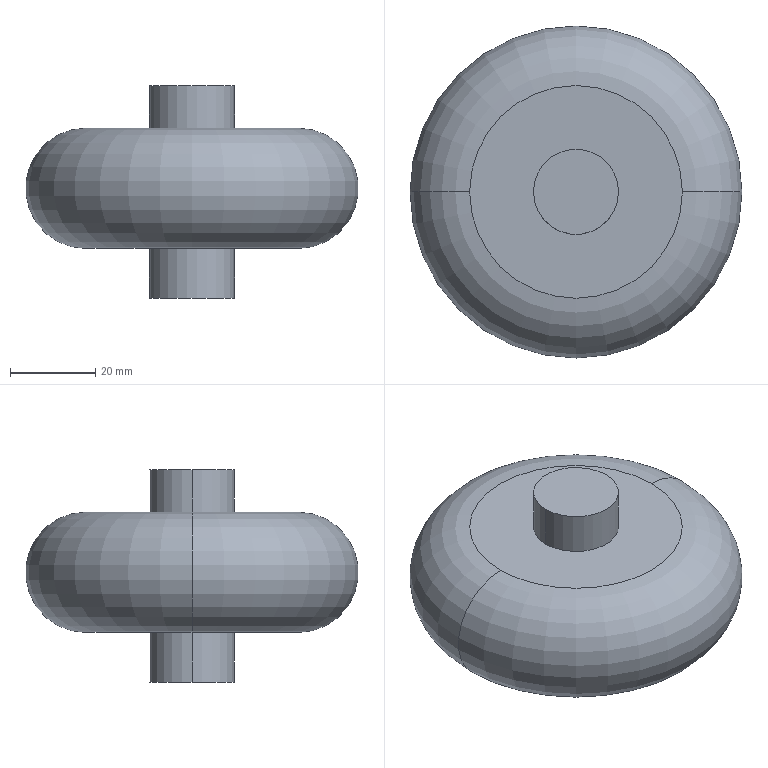Part | SolidWorks | features Extrusion 1, Revolution 1 | 1 solid | 10 faces | box 78.234 x 78.234 x 50 mm | volume 123364 mm3 | cylinder 4 | plane 4 | torus 2 | commonest cylinder face diameters 20 x4
STEP:
#1=CARTESIAN_POINT('',(10.,0.,25.));
#2=VERTEX_POINT('',#1);
#3=CARTESIAN_POINT('',(-10.,0.,25.));
#4=VERTEX_POINT('',#3);
#5=CARTESIAN_POINT('',(0.,0.,25.));
#6=DIRECTION('',(0.,0.,1.));
#7=DIRECTION('',(1.,0.,0.));
#8=AXIS2_PLACEMENT_3D('',#5,#6,#7);
#9=CIRCLE('',#8,10.);
#10=EDGE_CURVE('',#2,#4,#9,.T.);
#11=ORIENTED_EDGE('',*,*,#10,.F.);
#12=CARTESIAN_POINT('',(10.,0.,15.));
#13=VERTEX_POINT('',#12);
#14=CARTESIAN_POINT('',(10.,0.,25.));
#15=DIRECTION('',(0.,0.,-1.));
#16=VECTOR('',#15,1000.);
#17=LINE('',#14,#16);
#18=EDGE_CURVE('',#2,#13,#17,.T.);
#19=ORIENTED_EDGE('',*,*,#18,.T.);
#20=CARTESIAN_POINT('',(-10.,0.,15.));
#21=VERTEX_POINT('',#20);
#22=CARTESIAN_POINT('',(0.,0.,15.));
#23=DIRECTION('',(0.,0.,-1.));
#24=DIRECTION('',(-1.,0.,0.));
#25=AXIS2_PLACEMENT_3D('',#22,#23,#24);
#26=CIRCLE('',#25,10.);
#27=EDGE_CURVE('',#21,#13,#26,.T.);
#28=ORIENTED_EDGE('',*,*,#27,.F.);
#29=CARTESIAN_POINT('',(-10.,0.,25.));
#30=DIRECTION('',(0.,0.,-1.));
#31=VECTOR('',#30,1000.);
#32=LINE('',#29,#31);
#33=EDGE_CURVE('',#4,#21,#32,.T.);
#34=ORIENTED_EDGE('',*,*,#33,.F.);
#35=EDGE_LOOP('',(#11,#19,#28,#34));
#36=FACE_OUTER_BOUND('',#35,.T.);
#37=CARTESIAN_POINT('',(0.,0.,25.));
#38=DIRECTION('',(0.,0.,-1.));
#39=DIRECTION('',(-1.,0.,0.));
#40=AXIS2_PLACEMENT_3D('',#37,#38,#39);
#41=CYLINDRICAL_SURFACE('',#40,10.);
#42=ADVANCED_FACE('',(#36),#41,.T.);
#43=CARTESIAN_POINT('',(-24.991,0.,15.));
#44=VERTEX_POINT('',#43);
#45=CARTESIAN_POINT('',(24.991,0.,15.));
#46=VERTEX_POINT('',#45);
#47=CARTESIAN_POINT('',(-0.000000001,0.,15.));
#48=DIRECTION('',(0.,0.,-1.));
#49=DIRECTION('',(-1.,0.,0.));
#50=AXIS2_PLACEMENT_3D('',#47,#48,#49);
#51=CIRCLE('',#50,24.991);
#52=EDGE_CURVE('',#44,#46,#51,.T.);
#53=ORIENTED_EDGE('',*,*,#52,.T.);
#54=CARTESIAN_POINT('',(24.975,0.,-13.275));
#55=VERTEX_POINT('',#54);
#56=CARTESIAN_POINT('',(24.979,0.,0.8623));
#57=DIRECTION('',(0.,1.,0.));
#58=DIRECTION('',(-1.,0.,0.));
#59=AXIS2_PLACEMENT_3D('',#56,#57,#58);
#60=CIRCLE('',#59,14.138);
#61=EDGE_CURVE('',#46,#55,#60,.T.);
#62=ORIENTED_EDGE('',*,*,#61,.T.);
#63=CARTESIAN_POINT('',(-24.975,0.,-13.275));
#64=VERTEX_POINT('',#63);
#65=CARTESIAN_POINT('',(-0.000000001,0.,-13.275));
#66=DIRECTION('',(0.,0.,-1.));
#67=DIRECTION('',(-1.,0.,0.));
#68=AXIS2_PLACEMENT_3D('',#65,#66,#67);
#69=CIRCLE('',#68,24.975);
#70=EDGE_CURVE('',#64,#55,#69,.T.);
#71=ORIENTED_EDGE('',*,*,#70,.F.);
#72=CARTESIAN_POINT('',(-24.979,0.,0.8623));
#73=DIRECTION('',(0.,-1.,0.));
#74=DIRECTION('',(0.,0.,-1.));
#75=AXIS2_PLACEMENT_3D('',#72,#73,#74);
#76=CIRCLE('',#75,14.138);
#77=EDGE_CURVE('',#44,#64,#76,.T.);
#78=ORIENTED_EDGE('',*,*,#77,.F.);
#79=EDGE_LOOP('',(#53,#62,#71,#78));
#80=FACE_OUTER_BOUND('',#79,.T.);
#81=CARTESIAN_POINT('',(-0.000000001,0.,0.8623));
#82=DIRECTION('',(0.,0.,-1.));
#83=DIRECTION('',(-1.,0.,0.));
#84=AXIS2_PLACEMENT_3D('',#81,#82,#83);
#85=TOROIDAL_SURFACE('',#84,24.979,14.138);
#86=ADVANCED_FACE('',(#80),#85,.T.);
#87=CARTESIAN_POINT('',(10.,0.,-13.275));
#88=VERTEX_POINT('',#87);
#89=CARTESIAN_POINT('',(-10.,0.,-13.275));
#90=VERTEX_POINT('',#89);
#91=CARTESIAN_POINT('',(0.,0.,-13.275));
#92=DIRECTION('',(0.,0.,1.));
#93=DIRECTION('',(1.,0.,0.));
#94=AXIS2_PLACEMENT_3D('',#91,#92,#93);
#95=CIRCLE('',#94,10.);
#96=EDGE_CURVE('',#88,#90,#95,.T.);
#97=ORIENTED_EDGE('',*,*,#96,.F.);
#98=CARTESIAN_POINT('',(10.,0.,-25.));
#99=VERTEX_POINT('',#98);
#100=CARTESIAN_POINT('',(10.,0.,25.));
#101=DIRECTION('',(0.,0.,-1.));
#102=VECTOR('',#101,1000.);
#103=LINE('',#100,#102);
#104=EDGE_CURVE('',#88,#99,#103,.T.);
#105=ORIENTED_EDGE('',*,*,#104,.T.);
#106=CARTESIAN_POINT('',(-10.,0.,-25.));
#107=VERTEX_POINT('',#106);
#108=CARTESIAN_POINT('',(0.,0.,-25.));
#109=DIRECTION('',(0.,0.,1.));
#110=DIRECTION('',(1.,0.,0.));
#111=AXIS2_PLACEMENT_3D('',#108,#109,#110);
#112=CIRCLE('',#111,10.);
#113=EDGE_CURVE('',#99,#107,#112,.T.);
#114=ORIENTED_EDGE('',*,*,#113,.T.);
#115=CARTESIAN_POINT('',(-10.,0.,25.));
#116=DIRECTION('',(0.,0.,-1.));
#117=VECTOR('',#116,1000.);
#118=LINE('',#115,#117);
#119=EDGE_CURVE('',#90,#107,#118,.T.);
#120=ORIENTED_EDGE('',*,*,#119,.F.);
#121=EDGE_LOOP('',(#97,#105,#114,#120));
#122=FACE_OUTER_BOUND('',#121,.T.);
#123=CARTESIAN_POINT('',(0.,0.,25.));
#124=DIRECTION('',(0.,0.,-1.));
#125=DIRECTION('',(-1.,0.,0.));
#126=AXIS2_PLACEMENT_3D('',#123,#124,#125);
#127=CYLINDRICAL_SURFACE('',#126,10.);
#128=ADVANCED_FACE('',(#122),#127,.T.);
#129=ORIENTED_EDGE('',*,*,#104,.F.);
#130=CARTESIAN_POINT('',(0.,0.,-13.275));
#131=DIRECTION('',(0.,0.,1.));
#132=DIRECTION('',(1.,0.,0.));
#133=AXIS2_PLACEMENT_3D('',#130,#131,#132);
#134=CIRCLE('',#133,10.);
#135=EDGE_CURVE('',#90,#88,#134,.T.);
#136=ORIENTED_EDGE('',*,*,#135,.F.);
#137=ORIENTED_EDGE('',*,*,#119,.T.);
#138=CARTESIAN_POINT('',(0.,0.,-25.));
#139=DIRECTION('',(0.,0.,1.));
#140=DIRECTION('',(1.,0.,0.));
#141=AXIS2_PLACEMENT_3D('',#138,#139,#140);
#142=CIRCLE('',#141,10.);
#143=EDGE_CURVE('',#107,#99,#142,.T.);
#144=ORIENTED_EDGE('',*,*,#143,.T.);
#145=EDGE_LOOP('',(#129,#136,#137,#144));
#146=FACE_OUTER_BOUND('',#145,.T.);
#147=CARTESIAN_POINT('',(0.,0.,25.));
#148=DIRECTION('',(0.,0.,-1.));
#149=DIRECTION('',(-1.,0.,0.));
#150=AXIS2_PLACEMENT_3D('',#147,#148,#149);
#151=CYLINDRICAL_SURFACE('',#150,10.);
#152=ADVANCED_FACE('',(#146),#151,.T.);
#153=ORIENTED_EDGE('',*,*,#143,.F.);
#154=ORIENTED_EDGE('',*,*,#113,.F.);
#155=EDGE_LOOP('',(#153,#154));
#156=FACE_OUTER_BOUND('',#155,.T.);
#157=CARTESIAN_POINT('',(0.,0.,-25.));
#158=DIRECTION('',(0.,0.,1.));
#159=DIRECTION('',(1.,0.,0.));
#160=AXIS2_PLACEMENT_3D('',#157,#158,#159);
#161=PLANE('',#160);
#162=ADVANCED_FACE('',(#156),#161,.F.);
#163=ORIENTED_EDGE('',*,*,#135,.T.);
#164=ORIENTED_EDGE('',*,*,#96,.T.);
#165=EDGE_LOOP('',(#163,#164));
#166=FACE_BOUND('',#165,.T.);
#167=ORIENTED_EDGE('',*,*,#70,.T.);
#168=CARTESIAN_POINT('',(-0.000000001,0.,-13.275));
#169=DIRECTION('',(0.,0.,-1.));
#170=DIRECTION('',(-1.,0.,0.));
#171=AXIS2_PLACEMENT_3D('',#168,#169,#170);
#172=CIRCLE('',#171,24.975);
#173=EDGE_CURVE('',#55,#64,#172,.T.);
#174=ORIENTED_EDGE('',*,*,#173,.T.);
#175=EDGE_LOOP('',(#167,#174));
#176=FACE_OUTER_BOUND('',#175,.T.);
#177=CARTESIAN_POINT('',(0.,0.,-13.275));
#178=DIRECTION('',(0.,0.,1.));
#179=DIRECTION('',(1.,0.,0.));
#180=AXIS2_PLACEMENT_3D('',#177,#178,#179);
#181=PLANE('',#180);
#182=ADVANCED_FACE('',(#166,#176),#181,.F.);
#183=ORIENTED_EDGE('',*,*,#61,.F.);
#184=CARTESIAN_POINT('',(-0.000000001,0.,15.));
#185=DIRECTION('',(0.,0.,-1.));
#186=DIRECTION('',(-1.,0.,0.));
#187=AXIS2_PLACEMENT_3D('',#184,#185,#186);
#188=CIRCLE('',#187,24.991);
#189=EDGE_CURVE('',#46,#44,#188,.T.);
#190=ORIENTED_EDGE('',*,*,#189,.T.);
#191=ORIENTED_EDGE('',*,*,#77,.T.);
#192=ORIENTED_EDGE('',*,*,#173,.F.);
#193=EDGE_LOOP('',(#183,#190,#191,#192));
#194=FACE_OUTER_BOUND('',#193,.T.);
#195=CARTESIAN_POINT('',(-0.000000001,0.,0.8623));
#196=DIRECTION('',(0.,0.,-1.));
#197=DIRECTION('',(-1.,0.,0.));
#198=AXIS2_PLACEMENT_3D('',#195,#196,#197);
#199=TOROIDAL_SURFACE('',#198,24.979,14.138);
#200=ADVANCED_FACE('',(#194),#199,.T.);
#201=ORIENTED_EDGE('',*,*,#27,.T.);
#202=CARTESIAN_POINT('',(0.,0.,15.));
#203=DIRECTION('',(0.,0.,-1.));
#204=DIRECTION('',(-1.,0.,0.));
#205=AXIS2_PLACEMENT_3D('',#202,#203,#204);
#206=CIRCLE('',#205,10.);
#207=EDGE_CURVE('',#13,#21,#206,.T.);
#208=ORIENTED_EDGE('',*,*,#207,.T.);
#209=EDGE_LOOP('',(#201,#208));
#210=FACE_BOUND('',#209,.T.);
#211=ORIENTED_EDGE('',*,*,#52,.F.);
#212=ORIENTED_EDGE('',*,*,#189,.F.);
#213=EDGE_LOOP('',(#211,#212));
#214=FACE_OUTER_BOUND('',#213,.T.);
#215=CARTESIAN_POINT('',(0.,0.,15.));
#216=DIRECTION('',(0.,0.,-1.));
#217=DIRECTION('',(-1.,0.,0.));
#218=AXIS2_PLACEMENT_3D('',#215,#216,#217);
#219=PLANE('',#218);
#220=ADVANCED_FACE('',(#210,#214),#219,.F.);
#221=CARTESIAN_POINT('',(0.,0.,25.));
#222=DIRECTION('',(0.,0.,1.));
#223=DIRECTION('',(1.,0.,0.));
#224=AXIS2_PLACEMENT_3D('',#221,#222,#223);
#225=CIRCLE('',#224,10.);
#226=EDGE_CURVE('',#4,#2,#225,.T.);
#227=ORIENTED_EDGE('',*,*,#226,.T.);
#228=ORIENTED_EDGE('',*,*,#10,.T.);
#229=EDGE_LOOP('',(#227,#228));
#230=FACE_OUTER_BOUND('',#229,.T.);
#231=CARTESIAN_POINT('',(0.,0.,25.));
#232=DIRECTION('',(0.,0.,1.));
#233=DIRECTION('',(1.,0.,0.));
#234=AXIS2_PLACEMENT_3D('',#231,#232,#233);
#235=PLANE('',#234);
#236=ADVANCED_FACE('',(#230),#235,.T.);
#237=ORIENTED_EDGE('',*,*,#18,.F.);
#238=ORIENTED_EDGE('',*,*,#226,.F.);
#239=ORIENTED_EDGE('',*,*,#33,.T.);
#240=ORIENTED_EDGE('',*,*,#207,.F.);
#241=EDGE_LOOP('',(#237,#238,#239,#240));
#242=FACE_OUTER_BOUND('',#241,.T.);
#243=CARTESIAN_POINT('',(0.,0.,25.));
#244=DIRECTION('',(0.,0.,-1.));
#245=DIRECTION('',(-1.,0.,0.));
#246=AXIS2_PLACEMENT_3D('',#243,#244,#245);
#247=CYLINDRICAL_SURFACE('',#246,10.);
#248=ADVANCED_FACE('',(#242),#247,.T.);
#249=CLOSED_SHELL('',(#42,#86,#128,#152,#162,#182,#200,#220,#236,#248));
#250=MANIFOLD_SOLID_BREP('',#249);
#251=CARTESIAN_POINT('',(0.,0.,0.));
#252=DIRECTION('',(0.,0.,1.));
#253=DIRECTION('',(1.,0.,0.));
#254=AXIS2_PLACEMENT_3D('',#251,#252,#253);
#255=(LENGTH_UNIT()NAMED_UNIT(*)SI_UNIT(.MILLI.,.METRE.));
#256=UNCERTAINTY_MEASURE_WITH_UNIT(LENGTH_MEASURE(0.00001),#255,'','');
#257=(NAMED_UNIT(*)PLANE_ANGLE_UNIT()SI_UNIT($,.RADIAN.));
#258=(NAMED_UNIT(*)SI_UNIT($,.STERADIAN.)SOLID_ANGLE_UNIT());
#259=(GEOMETRIC_REPRESENTATION_CONTEXT(3)GLOBAL_UNCERTAINTY_ASSIGNED_CONTEXT((#256))GLOBAL_UNIT_ASSIGNED_CONTEXT((#255,#257,#258))REPRESENTATION_CONTEXT('',''));
#260=ADVANCED_BREP_SHAPE_REPRESENTATION('',(#250,#254),#259);